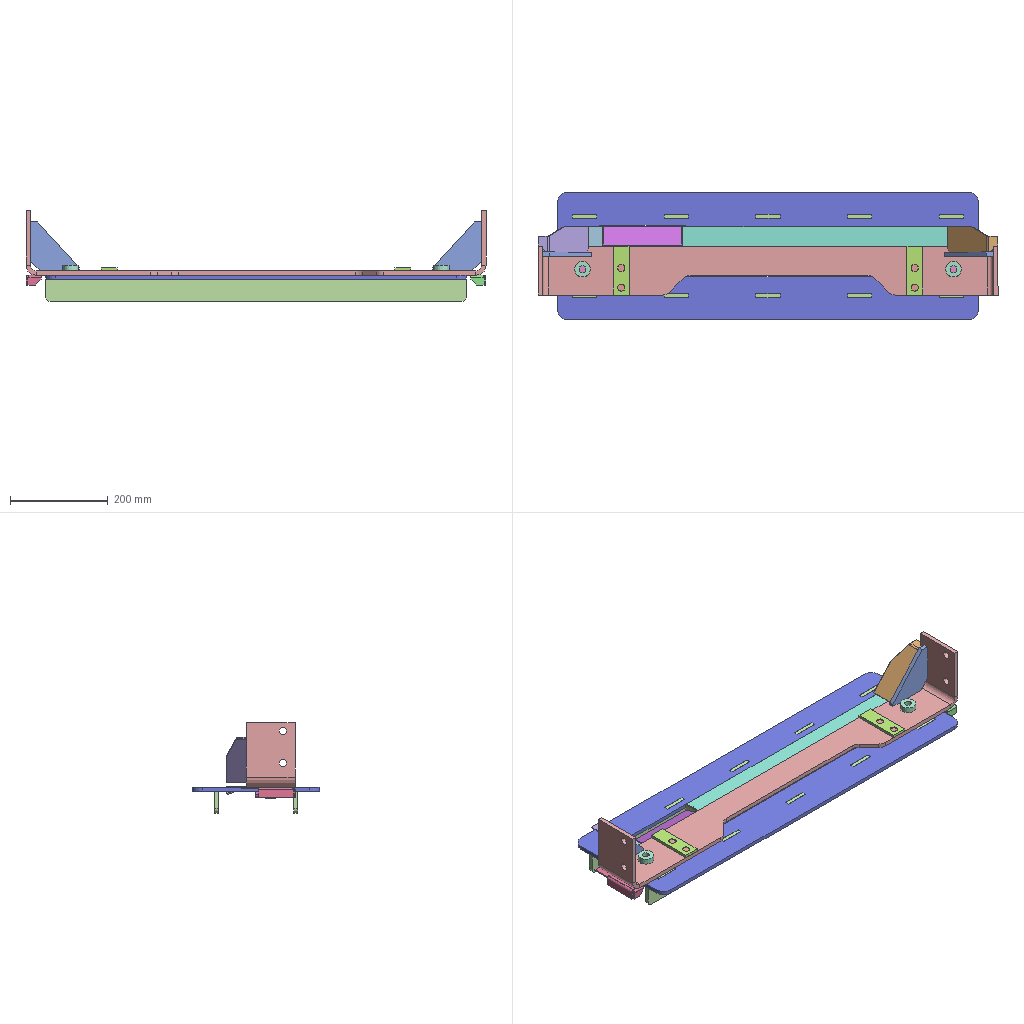Assembly | SolidWorks | 17 different items | 26 placed | box 940 x 260 x 185 mm
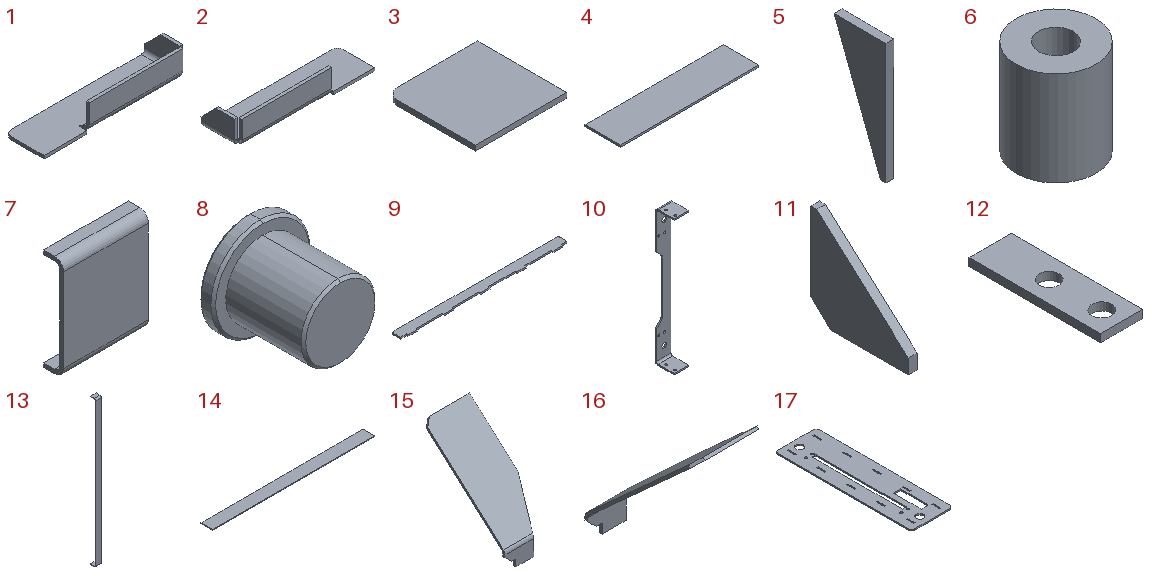Parts list (item | quantity | size | volume | features):
1 | x1 | 110 x 30 x 20 mm | 10965 mm3 | features Chamfer 1, EdgeFlange 1, FlatPattern 1, SMBaseFlange 1, SheetMetal 1
2 | x1 | 110 x 30 x 20 mm | 10965 mm3 | features Chamfer 1, EdgeFlange 1, FlatPattern 1, SMBaseFlange 1, SheetMetal 1
3 | x1 | 41 x 40 x 2.3 mm | 3760 mm3 | features FlatPattern 1, SMBaseFlange 1, SheetMetal 1
4 | x1 | 165 x 42 x 2.3 mm | 15939 mm3 | features FlatPattern 1, SMBaseFlange 1, SheetMetal 1
5 | x2 | 2.3 x 15 x 35 mm | 668.15 mm3 | features FlatPattern 1, SMBaseFlange 1, SheetMetal 1
6 | x2 | 32 x 32 x 38 mm | 24712 mm3 | features Extrusion 1, HoleWzd 1
7 | x2 | 50 x 11.8 x 60 mm | 8675 mm3 | features FlatPattern 1, SMBaseFlange 1, SheetMetal 1
8 | x4 | 20 x 18.7 x 20 mm | 3696 mm3 | features Chamfer 1, Revolution 1
9 | x2 | 860 x 52.5 x 8 mm | 324257 mm3 | features FlatPattern 1, SMBaseFlange 1, SheetMetal 1
10 | x1 | 100 x 132 x 940 mm | 876071 mm3 | features ICE 2, Fillet 1, FlatPattern 1, SMBaseFlange 1, SheetMetal 1
11 | x2 | 9 x 100 x 100 mm | 52245 mm3 | features FlatPattern 1, SMBaseFlange 1, SheetMetal 1
12 | x2 | 32 x 100 x 6 mm | 17079 mm3 | features FlatPattern 1, SMBaseFlange 1, SheetMetal 1
13 | x1 | 22 x 20 x 560 mm | 29947 mm3 | features FlatPattern 1, SMBaseFlange 1, SheetMetal 1
14 | x1 | 554 x 40 x 2.3 mm | 50956 mm3 | features FlatPattern 1, SMBaseFlange 1, SheetMetal 1
15 | x1 | 52 x 93.043 x 102.735 mm | 14624 mm3 | features ICE 2, Chamfer 1, FlatPattern 1, SMBaseFlange 1, SheetMetal 1
16 | x1 | 52 x 93.043 x 102.735 mm | 14624 mm3 | features ICE 2, Chamfer 1, FlatPattern 1, SMBaseFlange 1, SheetMetal 1
17 | x1 | 260 x 860 x 8 mm | 1544579 mm3 | features FlatPattern 1, SMBaseFlange 1, SheetMetal 1
Mates (type | each side: item.copy, entity, surface, feature):
Coincident | 10.1 face plane Base-Flange1 | 11.1 face plane Base-Flange1 | 2 times
DistanceDim | 10.1 face plane Base-Flange1 | 11.1 face plane Base-Flange1
Coincident | 10.1 face plane Base-Flange1 | 11.2 face plane Base-Flange1 | 2 times
DistanceDim | 10.1 face plane Base-Flange1 | 11.2 face plane Base-Flange1
Coincident | 10.1 face plane Base-Flange1 | 12.1 face plane Base-Flange1
Concentric | 10.1 face cylinder Cut-Extrude1 | 12.1 face cylinder Base-Flange1 | 2 times
Coincident | 10.1 face plane Base-Flange1 | 12.2 face plane Base-Flange1
Concentric | 10.1 face cylinder Cut-Extrude1 | 12.2 face cylinder Base-Flange1 | 2 times
Coincident | 10.1 face plane Base-Flange1 | 13.1 face plane Base-Flange1
DistanceDim | 10.1 face plane Base-Flange1 | 13.1 face plane Base-Flange1
Coincident | 10.1 face plane Cut-Extrude1 | 13.1 face plane Base-Flange1
Coincident | 14.1 face plane Base-Flange1 | 10.1 face plane Base-Flange1
Coincident | 10.1 face plane Base-Flange1 | 14.1 face plane Base-Flange1
DistanceDim | 10.1 face plane Base-Flange1 | 14.1 face plane Base-Flange1
Coincident | 11.2 face plane Base-Flange1 | 15.1 face plane Base-Flange1
Coincident | 10.1 face plane Base-Flange1 | 15.1 face plane Cut-Extrude3
DistanceDim | 10.1 face plane Base-Flange1 | 15.1 face plane Base-Flange1
Coincident | 10.1 face plane Base-Flange1 | 16.1 face plane Cut-Extrude3
DistanceDim | 10.1 face plane Base-Flange1 | 16.1 face plane Base-Flange1
Coincident | 11.1 face plane Base-Flange1 | 16.1 face plane Base-Flange1
Coincident | 10.1 face plane Base-Flange1 | 1.1 face plane Base-Flange1
DistanceDim | 1.1 face plane Edge-Flange1 | 10.1 face plane Base-Flange1
Coincident | 10.1 face plane Base-Flange1 | 1.1 face plane Edge-Flange1
Coincident | 10.1 face plane Base-Flange1 | 2.1 face plane Base-Flange1
Coincident | 10.1 face plane Base-Flange1 | 2.1 face plane Edge-Flange1
DistanceDim | 10.1 face plane Base-Flange1 | 2.1 face plane Edge-Flange1
Coincident | 10.1 face plane Base-Flange1 | 3.1 face plane Base-Flange1 | 2 times
DistanceDim | 3.1 face plane Base-Flange1 | 10.1 face plane Base-Flange1
Coincident | 14.1 face plane Base-Flange1 | 5.1 face plane Base-Flange1 | 3 times
Coincident | 3.1 face plane Base-Flange1 | 5.2 face plane Base-Flange1 | 3 times
Coincident | 5.1 face plane Base-Flange1 | 4.1 face plane Base-Flange1 | 2 times
Coincident | 5.1 edge | 4.1 edge
Concentric | 10.1 face cylinder Cut-Extrude1 | 6.1 face cylinder Boss-Extrude1
DistanceDim | 6.1 face plane Boss-Extrude1 | 10.1 face plane Base-Flange1
Parallel | 10.1 face plane Base-Flange1 | 6.1 plane
Concentric | 10.1 face cylinder Cut-Extrude1 | 6.2 face cylinder Boss-Extrude1
DistanceDim | 6.2 face plane Boss-Extrude1 | 10.1 face plane Base-Flange1
Parallel | 10.1 face plane Base-Flange1 | 6.2 plane
Coincident | 8.1 face plane Revolve1 | 8.2 face plane Revolve1
Coincident | 8.1 face plane Revolve1 | 8.3 face plane Revolve1
Coincident | 8.3 face plane Revolve1 | 8.4 face plane Revolve1
InPlace | 10.1 face plane Base-Flange1 | 17.1 plane
InPlace | 9.1 plane | assembly plane
DistanceDim | 10.1 face plane Base-Flange1 | 7.1 face plane Base-Flange1